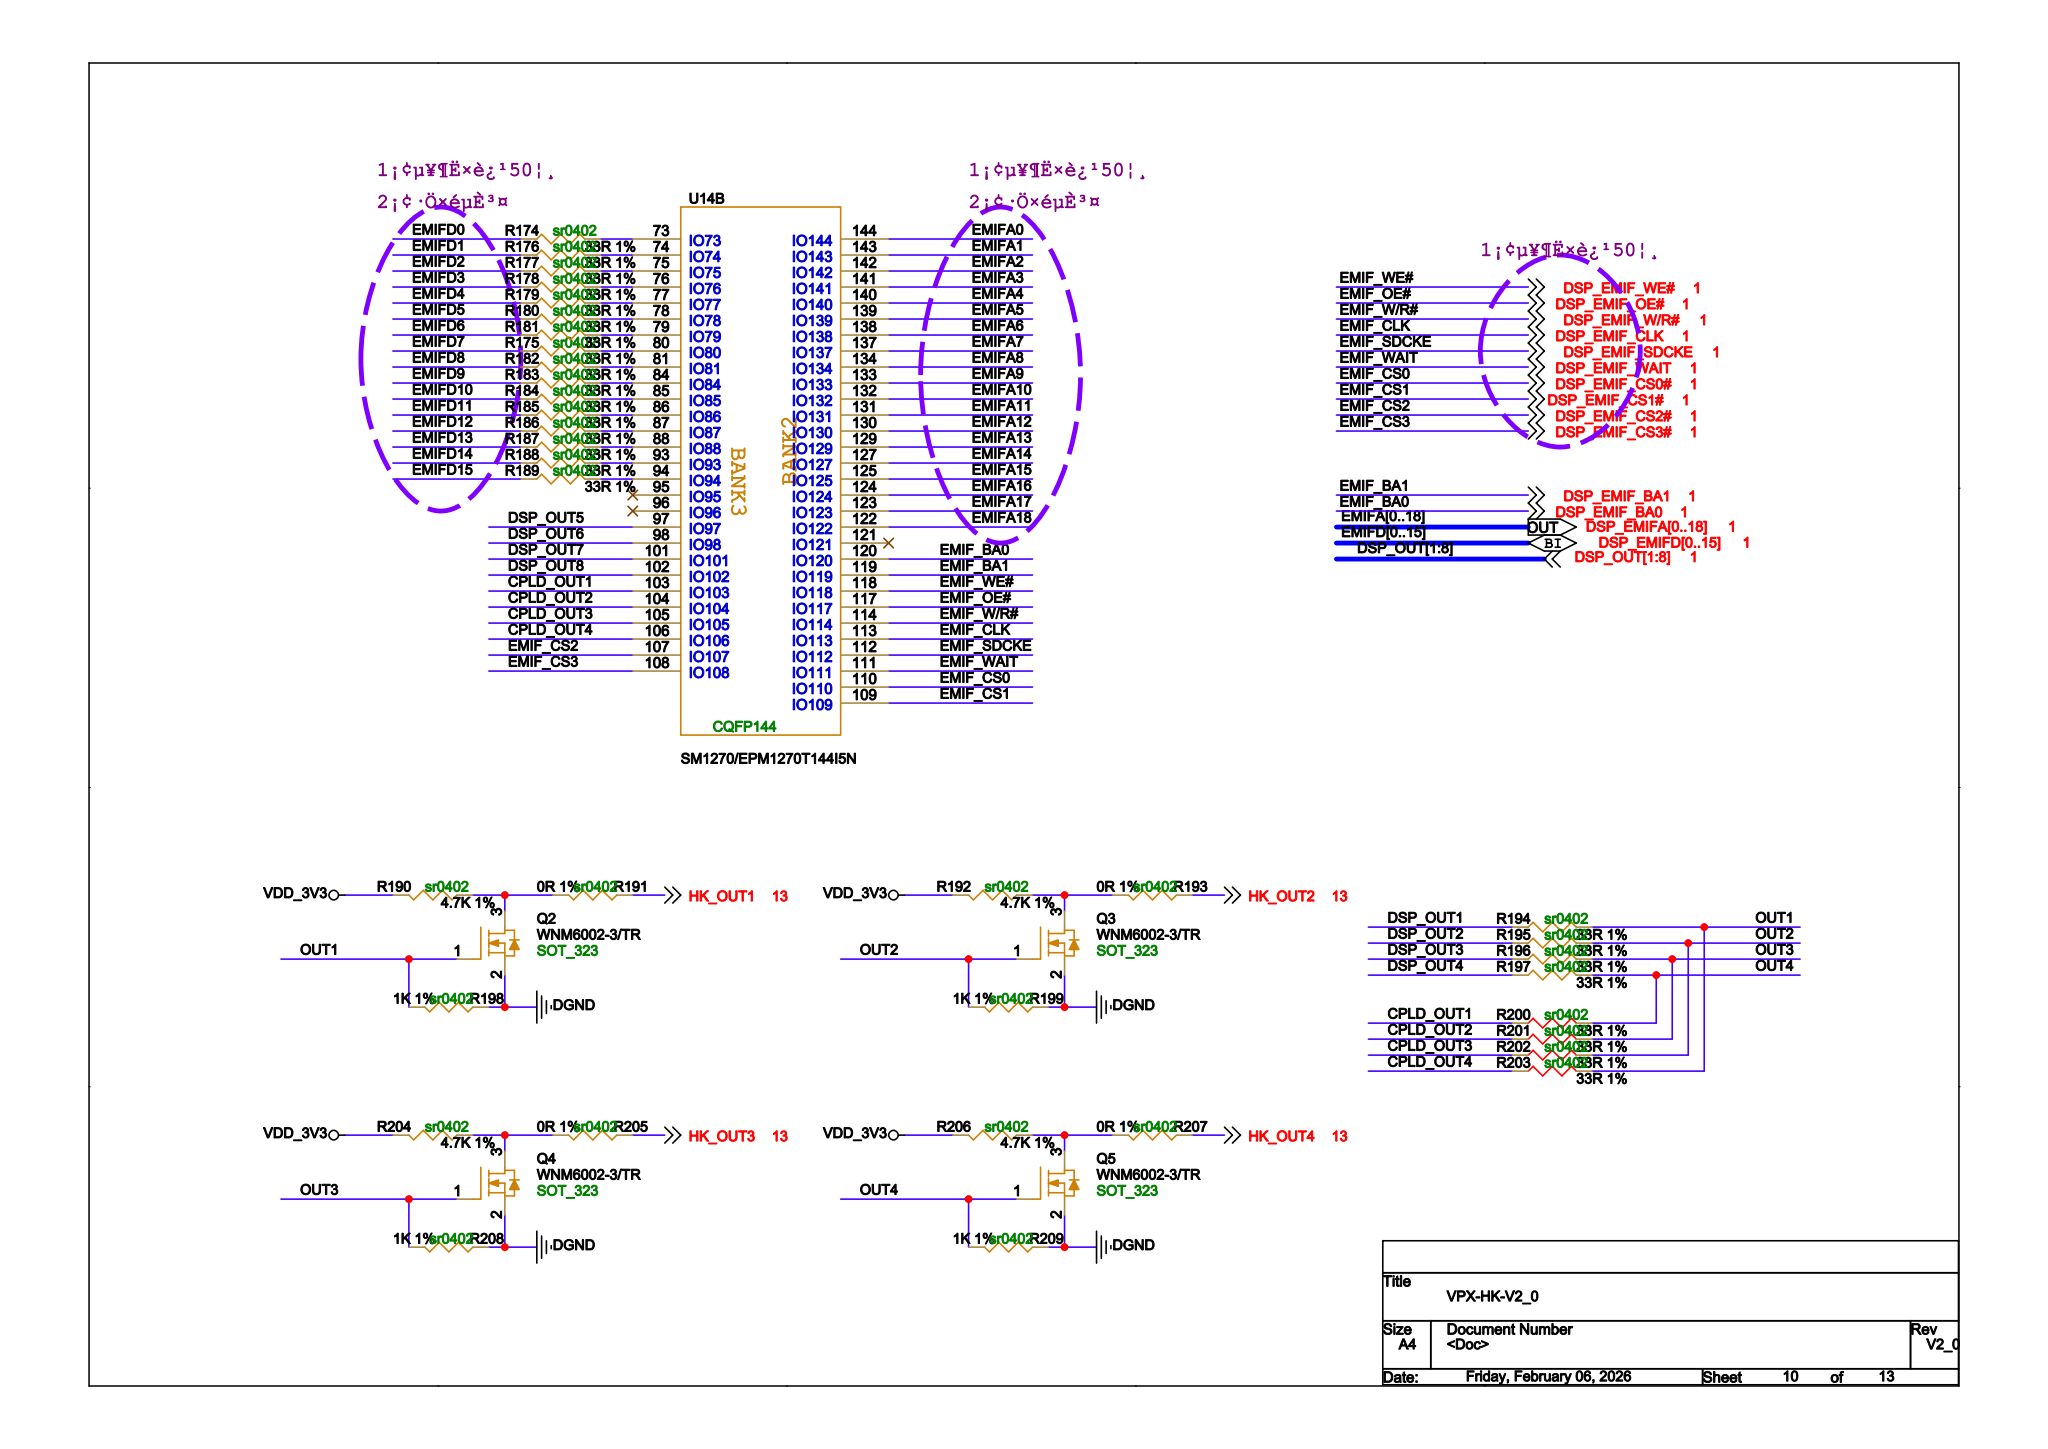Circuit board | Cadence Allegro | 598 parts | 541 nets | one sheet of the schematic
Parts on this sheet (reference | value | footprint):
Q2 | WNM6002-3/TR | SOT_323
Q3 | WNM6002-3/TR | SOT_323
Q4 | WNM6002-3/TR | SOT_323
Q5 | WNM6002-3/TR | SOT_323
R174 | 33R 1% | SR0402
R175 | 33R 1% | SR0402
R176 | 33R 1% | SR0402
R177 | 33R 1% | SR0402
R178 | 33R 1% | SR0402
R179 | 33R 1% | SR0402
R180 | 33R 1% | SR0402
R181 | 33R 1% | SR0402
R182 | 33R 1% | SR0402
R183 | 33R 1% | SR0402
R184 | 33R 1% | SR0402
R185 | 33R 1% | SR0402
R186 | 33R 1% | SR0402
R187 | 33R 1% | SR0402
R188 | 33R 1% | SR0402
R189 | 33R 1% | SR0402
R190 | 4.7K 1% | SR0402
R192 | 4.7K 1% | SR0402
R194 | 33R 1% | SR0402
R195 | 33R 1% | SR0402
R196 | 33R 1% | SR0402
R197 | 33R 1% | SR0402
R200 | 33R 1% | SR0402
R201 | 33R 1% | SR0402
R202 | 33R 1% | SR0402
R203 | 33R 1% | SR0402
R204 | 4.7K 1% | SR0402
R206 | 4.7K 1% | SR0402
U14 | SM1270/EPM1270T144I5N | CQFP144
Nets of these parts (net: part-pin ...):
DGND: Q2-2 Q3-2 Q4-2 Q5-2 U14-10
DSP_OUT7: U14-101
DSP_OUT8: U14-102
CPLD_OUT1: R200-1 U14-103
CPLD_OUT2: R201-1 U14-104
CPLD_OUT3: R202-1 U14-105
CPLD_OUT4: R203-1 U14-106
DSP_EMIF_CS2#: U14-107
DSP_EMIF_CS3#: U14-108
DSP_EMIF_CS1#: U14-109
DSP_EMIF_CS0#: U14-110
DSP_EMIF_WAIT: U14-111
DSP_EMIF_SDCKE: U14-112
DSP_EMIF_CLK: U14-113
DSP_EMIF_W/R#: U14-114
DSP_EMIF_OE#: U14-117
DSP_EMIF_WE#: U14-118
DSP_EMIF_BA1: U14-119
DSP_EMIF_BA0: U14-120
N33543192: R174-2 U14-73
N33543189: R176-2 U14-74
N33543191: R177-2 U14-75
N33543180: R178-2 U14-76
N33543182: R179-2 U14-77
N33543186: R180-2 U14-78
N33543187: R181-2 U14-79
N33543194: R175-2 U14-80
N33543185: R182-2 U14-81
N33543184: R183-2 U14-84
N33543181: R184-2 U14-85
N33543193: R185-2 U14-86
N33543190: R186-2 U14-87
N33543183: R187-2 U14-88
N33543188: R188-2 U14-93
N33543195: R189-2 U14-94
DSP_OUT5: U14-97
DSP_OUT6: U14-98
VDD_3V3: R190-1 R192-1 R204-1 R206-1
N33548180: Q2-3 R190-2
OUT1: Q2-1 R194-2 R203-2
N33548524: Q3-3 R192-2
OUT2: Q3-1 R195-2 R202-2
N33548731: Q4-3 R204-2
OUT3: Q4-1 R196-2 R201-2
N33548903: Q5-3 R206-2
OUT4: Q5-1 R197-2 R200-2
DSP_EMIFD12: R186-1
DSP_EMIFD15: R189-1
DSP_OUT4: R197-1
DSP_EMIFD0: R174-1
DSP_EMIFD7: R175-1
DSP_EMIFD1: R176-1
DSP_EMIFD2: R177-1
DSP_EMIFD3: R178-1
DSP_EMIFD4: R179-1
DSP_EMIFD5: R180-1
DSP_EMIFD6: R181-1
DSP_EMIFD8: R182-1
DSP_EMIFD9: R183-1
DSP_EMIFD10: R184-1
DSP_EMIFD11: R185-1
DSP_EMIFD13: R187-1
DSP_EMIFD14: R188-1
DSP_OUT1: R194-1
DSP_OUT2: R195-1
DSP_OUT3: R196-1